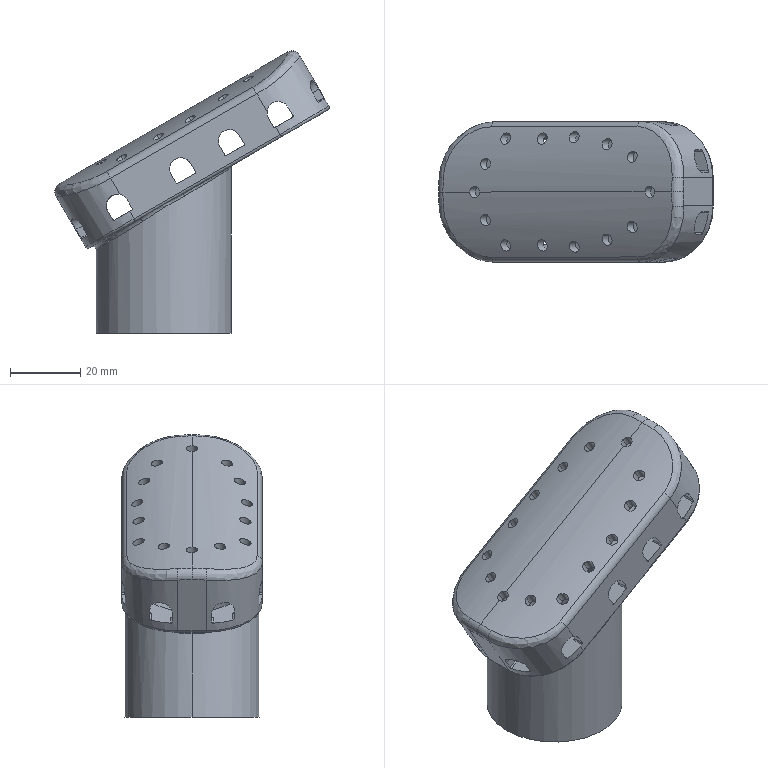Part | STEP file | RJWD-DY-010607_3D0001 | 1 solid | 176 faces | box 78.111 x 40 x 80.345 mm | volume 35899 mm3 | cylinder 104 | plane 40 | spline 18 | torus 12 | cone 2 | commonest cylinder face diameters 3.2 x28 0.8 x24 6.4 x18 8 x10 32 x6 1.6 x4